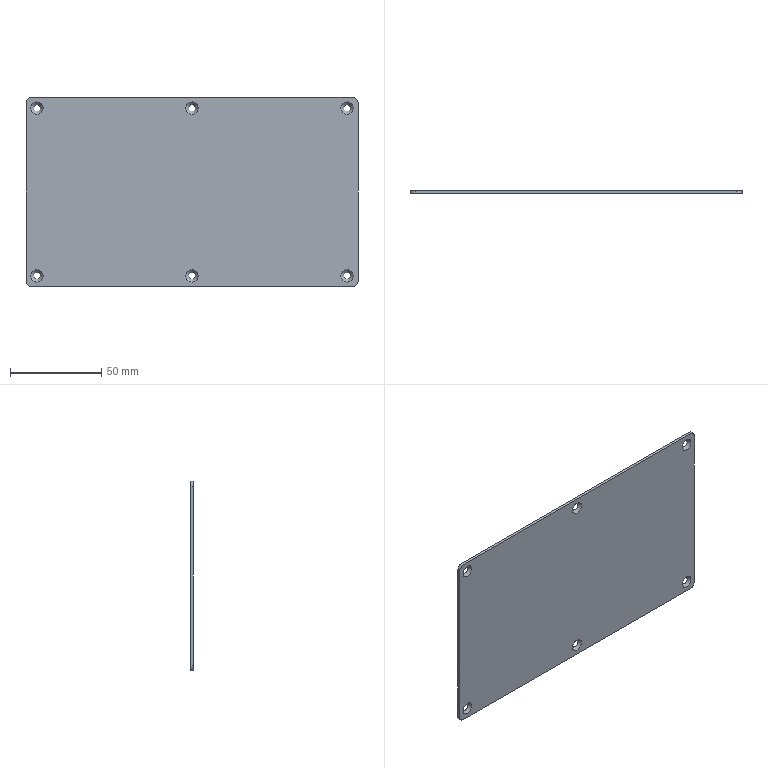Part | NX | 1 solid | 16 faces | box 182 x 1.5 x 104 mm | volume 28183 mm3 | plane 6 | cone 6 | cylinder 4 | commonest cylinder face diameters 6 x4
STEP:
#1=CARTESIAN_POINT('',(-85.,1.5,47.86));
#2=VERTEX_POINT('',#1);
#3=CARTESIAN_POINT('',(-85.,1.5,46.));
#4=DIRECTION('',(0.,1.,0.));
#5=DIRECTION('',(0.,0.,1.));
#6=AXIS2_PLACEMENT_3D('',#3,#4,#5);
#7=CIRCLE('',#6,1.86);
#8=EDGE_CURVE('',#2,#2,#7,.T.);
#9=ORIENTED_EDGE('',*,*,#8,.F.);
#10=EDGE_LOOP('',(#9));
#11=FACE_BOUND('',#10,.T.);
#12=CARTESIAN_POINT('',(-85.,1.5,-44.14));
#13=VERTEX_POINT('',#12);
#14=CARTESIAN_POINT('',(-85.,1.5,-46.));
#15=DIRECTION('',(0.,1.,0.));
#16=DIRECTION('',(0.,0.,1.));
#17=AXIS2_PLACEMENT_3D('',#14,#15,#16);
#18=CIRCLE('',#17,1.86);
#19=EDGE_CURVE('',#13,#13,#18,.T.);
#20=ORIENTED_EDGE('',*,*,#19,.F.);
#21=EDGE_LOOP('',(#20));
#22=FACE_BOUND('',#21,.T.);
#23=CARTESIAN_POINT('',(85.,1.5,-44.14));
#24=VERTEX_POINT('',#23);
#25=CARTESIAN_POINT('',(85.,1.5,-46.));
#26=DIRECTION('',(0.,1.,0.));
#27=DIRECTION('',(0.,0.,1.));
#28=AXIS2_PLACEMENT_3D('',#25,#26,#27);
#29=CIRCLE('',#28,1.86);
#30=EDGE_CURVE('',#24,#24,#29,.T.);
#31=ORIENTED_EDGE('',*,*,#30,.F.);
#32=EDGE_LOOP('',(#31));
#33=FACE_BOUND('',#32,.T.);
#34=CARTESIAN_POINT('',(0.,1.5,-44.14));
#35=VERTEX_POINT('',#34);
#36=CARTESIAN_POINT('',(0.,1.5,-46.));
#37=DIRECTION('',(0.,1.,0.));
#38=DIRECTION('',(0.,0.,1.));
#39=AXIS2_PLACEMENT_3D('',#36,#37,#38);
#40=CIRCLE('',#39,1.86);
#41=EDGE_CURVE('',#35,#35,#40,.T.);
#42=ORIENTED_EDGE('',*,*,#41,.F.);
#43=EDGE_LOOP('',(#42));
#44=FACE_BOUND('',#43,.T.);
#45=CARTESIAN_POINT('',(-88.,1.5,52.));
#46=VERTEX_POINT('',#45);
#47=CARTESIAN_POINT('',(88.,1.5,52.));
#48=VERTEX_POINT('',#47);
#49=CARTESIAN_POINT('',(-91.,1.5,52.));
#50=DIRECTION('',(1.,0.,0.));
#51=VECTOR('',#50,1000.);
#52=LINE('',#49,#51);
#53=EDGE_CURVE('',#46,#48,#52,.T.);
#54=ORIENTED_EDGE('',*,*,#53,.T.);
#55=CARTESIAN_POINT('',(91.,1.5,49.));
#56=VERTEX_POINT('',#55);
#57=CARTESIAN_POINT('',(88.,1.5,49.));
#58=DIRECTION('',(0.,1.,0.));
#59=DIRECTION('',(0.,0.,1.));
#60=AXIS2_PLACEMENT_3D('',#57,#58,#59);
#61=CIRCLE('',#60,3.);
#62=EDGE_CURVE('',#48,#56,#61,.T.);
#63=ORIENTED_EDGE('',*,*,#62,.T.);
#64=CARTESIAN_POINT('',(91.,1.5,-49.));
#65=VERTEX_POINT('',#64);
#66=CARTESIAN_POINT('',(91.,1.5,-52.));
#67=DIRECTION('',(0.,0.,-1.));
#68=VECTOR('',#67,1000.);
#69=LINE('',#66,#68);
#70=EDGE_CURVE('',#56,#65,#69,.T.);
#71=ORIENTED_EDGE('',*,*,#70,.T.);
#72=CARTESIAN_POINT('',(88.,1.5,-52.));
#73=VERTEX_POINT('',#72);
#74=CARTESIAN_POINT('',(88.,1.5,-49.));
#75=DIRECTION('',(0.,1.,0.));
#76=DIRECTION('',(0.,0.,1.));
#77=AXIS2_PLACEMENT_3D('',#74,#75,#76);
#78=CIRCLE('',#77,3.);
#79=EDGE_CURVE('',#65,#73,#78,.T.);
#80=ORIENTED_EDGE('',*,*,#79,.T.);
#81=CARTESIAN_POINT('',(-88.,1.5,-52.));
#82=VERTEX_POINT('',#81);
#83=CARTESIAN_POINT('',(-91.,1.5,-52.));
#84=DIRECTION('',(-1.,0.,0.));
#85=VECTOR('',#84,1000.);
#86=LINE('',#83,#85);
#87=EDGE_CURVE('',#73,#82,#86,.T.);
#88=ORIENTED_EDGE('',*,*,#87,.T.);
#89=CARTESIAN_POINT('',(-91.,1.5,-49.));
#90=VERTEX_POINT('',#89);
#91=CARTESIAN_POINT('',(-88.,1.5,-49.));
#92=DIRECTION('',(0.,1.,0.));
#93=DIRECTION('',(0.,0.,1.));
#94=AXIS2_PLACEMENT_3D('',#91,#92,#93);
#95=CIRCLE('',#94,3.);
#96=EDGE_CURVE('',#82,#90,#95,.T.);
#97=ORIENTED_EDGE('',*,*,#96,.T.);
#98=CARTESIAN_POINT('',(-91.,1.5,49.));
#99=VERTEX_POINT('',#98);
#100=CARTESIAN_POINT('',(-91.,1.5,-52.));
#101=DIRECTION('',(0.,0.,1.));
#102=VECTOR('',#101,1000.);
#103=LINE('',#100,#102);
#104=EDGE_CURVE('',#90,#99,#103,.T.);
#105=ORIENTED_EDGE('',*,*,#104,.T.);
#106=CARTESIAN_POINT('',(-88.,1.5,49.));
#107=DIRECTION('',(0.,1.,0.));
#108=DIRECTION('',(0.,0.,1.));
#109=AXIS2_PLACEMENT_3D('',#106,#107,#108);
#110=CIRCLE('',#109,3.);
#111=EDGE_CURVE('',#99,#46,#110,.T.);
#112=ORIENTED_EDGE('',*,*,#111,.T.);
#113=EDGE_LOOP('',(#54,#63,#71,#80,#88,#97,#105,#112));
#114=FACE_BOUND('',#113,.T.);
#115=CARTESIAN_POINT('',(0.,1.5,47.86));
#116=VERTEX_POINT('',#115);
#117=CARTESIAN_POINT('',(0.,1.5,46.));
#118=DIRECTION('',(0.,1.,0.));
#119=DIRECTION('',(0.,0.,1.));
#120=AXIS2_PLACEMENT_3D('',#117,#118,#119);
#121=CIRCLE('',#120,1.86);
#122=EDGE_CURVE('',#116,#116,#121,.T.);
#123=ORIENTED_EDGE('',*,*,#122,.F.);
#124=EDGE_LOOP('',(#123));
#125=FACE_BOUND('',#124,.T.);
#126=CARTESIAN_POINT('',(85.,1.5,47.86));
#127=VERTEX_POINT('',#126);
#128=CARTESIAN_POINT('',(85.,1.5,46.));
#129=DIRECTION('',(0.,1.,0.));
#130=DIRECTION('',(0.,0.,1.));
#131=AXIS2_PLACEMENT_3D('',#128,#129,#130);
#132=CIRCLE('',#131,1.86);
#133=EDGE_CURVE('',#127,#127,#132,.T.);
#134=ORIENTED_EDGE('',*,*,#133,.F.);
#135=EDGE_LOOP('',(#134));
#136=FACE_BOUND('',#135,.T.);
#137=CARTESIAN_POINT('',(0.,1.5,0.));
#138=DIRECTION('',(0.,1.,0.));
#139=DIRECTION('',(0.,0.,1.));
#140=AXIS2_PLACEMENT_3D('',#137,#138,#139);
#141=PLANE('',#140);
#142=ADVANCED_FACE('',(#11,#22,#33,#44,#114,#125,#136),#141,.T.);
#143=ORIENTED_EDGE('',*,*,#70,.F.);
#144=CARTESIAN_POINT('',(91.,0.,49.));
#145=VERTEX_POINT('',#144);
#146=CARTESIAN_POINT('',(91.,1.5,49.));
#147=DIRECTION('',(0.,-1.,0.));
#148=VECTOR('',#147,1000.);
#149=LINE('',#146,#148);
#150=EDGE_CURVE('',#56,#145,#149,.T.);
#151=ORIENTED_EDGE('',*,*,#150,.T.);
#152=CARTESIAN_POINT('',(91.,0.,-49.));
#153=VERTEX_POINT('',#152);
#154=CARTESIAN_POINT('',(91.,0.,-52.));
#155=DIRECTION('',(0.,0.,-1.));
#156=VECTOR('',#155,1000.);
#157=LINE('',#154,#156);
#158=EDGE_CURVE('',#145,#153,#157,.T.);
#159=ORIENTED_EDGE('',*,*,#158,.T.);
#160=CARTESIAN_POINT('',(91.,1.5,-49.));
#161=DIRECTION('',(0.,-1.,0.));
#162=VECTOR('',#161,1000.);
#163=LINE('',#160,#162);
#164=EDGE_CURVE('',#153,#65,#163,.F.);
#165=ORIENTED_EDGE('',*,*,#164,.T.);
#166=EDGE_LOOP('',(#143,#151,#159,#165));
#167=FACE_BOUND('',#166,.T.);
#168=CARTESIAN_POINT('',(91.,1.5,-52.));
#169=DIRECTION('',(-1.,0.,0.));
#170=DIRECTION('',(0.,0.,1.));
#171=AXIS2_PLACEMENT_3D('',#168,#169,#170);
#172=PLANE('',#171);
#173=ADVANCED_FACE('',(#167),#172,.F.);
#174=ORIENTED_EDGE('',*,*,#87,.F.);
#175=CARTESIAN_POINT('',(88.,0.,-52.));
#176=VERTEX_POINT('',#175);
#177=CARTESIAN_POINT('',(88.,1.5,-52.));
#178=DIRECTION('',(0.,-1.,0.));
#179=VECTOR('',#178,1000.);
#180=LINE('',#177,#179);
#181=EDGE_CURVE('',#73,#176,#180,.T.);
#182=ORIENTED_EDGE('',*,*,#181,.T.);
#183=CARTESIAN_POINT('',(-88.,0.,-52.));
#184=VERTEX_POINT('',#183);
#185=CARTESIAN_POINT('',(-91.,0.,-52.));
#186=DIRECTION('',(-1.,0.,0.));
#187=VECTOR('',#186,1000.);
#188=LINE('',#185,#187);
#189=EDGE_CURVE('',#176,#184,#188,.T.);
#190=ORIENTED_EDGE('',*,*,#189,.T.);
#191=CARTESIAN_POINT('',(-88.,1.5,-52.));
#192=DIRECTION('',(0.,-1.,0.));
#193=VECTOR('',#192,1000.);
#194=LINE('',#191,#193);
#195=EDGE_CURVE('',#184,#82,#194,.F.);
#196=ORIENTED_EDGE('',*,*,#195,.T.);
#197=EDGE_LOOP('',(#174,#182,#190,#196));
#198=FACE_BOUND('',#197,.T.);
#199=CARTESIAN_POINT('',(-91.,1.5,-52.));
#200=DIRECTION('',(0.,0.,1.));
#201=DIRECTION('',(1.,0.,0.));
#202=AXIS2_PLACEMENT_3D('',#199,#200,#201);
#203=PLANE('',#202);
#204=ADVANCED_FACE('',(#198),#203,.F.);
#205=CARTESIAN_POINT('',(-91.,0.,-49.));
#206=VERTEX_POINT('',#205);
#207=CARTESIAN_POINT('',(-91.,0.,49.));
#208=VERTEX_POINT('',#207);
#209=CARTESIAN_POINT('',(-91.,0.,-52.));
#210=DIRECTION('',(0.,0.,1.));
#211=VECTOR('',#210,1000.);
#212=LINE('',#209,#211);
#213=EDGE_CURVE('',#206,#208,#212,.T.);
#214=ORIENTED_EDGE('',*,*,#213,.T.);
#215=CARTESIAN_POINT('',(-91.,1.5,49.));
#216=DIRECTION('',(0.,-1.,0.));
#217=VECTOR('',#216,1000.);
#218=LINE('',#215,#217);
#219=EDGE_CURVE('',#208,#99,#218,.F.);
#220=ORIENTED_EDGE('',*,*,#219,.T.);
#221=ORIENTED_EDGE('',*,*,#104,.F.);
#222=CARTESIAN_POINT('',(-91.,1.5,-49.));
#223=DIRECTION('',(0.,-1.,0.));
#224=VECTOR('',#223,1000.);
#225=LINE('',#222,#224);
#226=EDGE_CURVE('',#90,#206,#225,.T.);
#227=ORIENTED_EDGE('',*,*,#226,.T.);
#228=EDGE_LOOP('',(#214,#220,#221,#227));
#229=FACE_BOUND('',#228,.T.);
#230=CARTESIAN_POINT('',(-91.,1.5,-52.));
#231=DIRECTION('',(1.,0.,0.));
#232=DIRECTION('',(0.,0.,-1.));
#233=AXIS2_PLACEMENT_3D('',#230,#231,#232);
#234=PLANE('',#233);
#235=ADVANCED_FACE('',(#229),#234,.F.);
#236=CARTESIAN_POINT('',(-88.,0.,52.));
#237=VERTEX_POINT('',#236);
#238=CARTESIAN_POINT('',(88.,0.,52.));
#239=VERTEX_POINT('',#238);
#240=CARTESIAN_POINT('',(-91.,0.,52.));
#241=DIRECTION('',(1.,0.,0.));
#242=VECTOR('',#241,1000.);
#243=LINE('',#240,#242);
#244=EDGE_CURVE('',#237,#239,#243,.T.);
#245=ORIENTED_EDGE('',*,*,#244,.T.);
#246=CARTESIAN_POINT('',(88.,1.5,52.));
#247=DIRECTION('',(0.,-1.,0.));
#248=VECTOR('',#247,1000.);
#249=LINE('',#246,#248);
#250=EDGE_CURVE('',#239,#48,#249,.F.);
#251=ORIENTED_EDGE('',*,*,#250,.T.);
#252=ORIENTED_EDGE('',*,*,#53,.F.);
#253=CARTESIAN_POINT('',(-88.,1.5,52.));
#254=DIRECTION('',(0.,-1.,0.));
#255=VECTOR('',#254,1000.);
#256=LINE('',#253,#255);
#257=EDGE_CURVE('',#46,#237,#256,.T.);
#258=ORIENTED_EDGE('',*,*,#257,.T.);
#259=EDGE_LOOP('',(#245,#251,#252,#258));
#260=FACE_BOUND('',#259,.T.);
#261=CARTESIAN_POINT('',(-91.,1.5,52.));
#262=DIRECTION('',(0.,0.,-1.));
#263=DIRECTION('',(-1.,0.,0.));
#264=AXIS2_PLACEMENT_3D('',#261,#262,#263);
#265=PLANE('',#264);
#266=ADVANCED_FACE('',(#260),#265,.F.);
#267=CARTESIAN_POINT('',(-85.,0.,42.64));
#268=VERTEX_POINT('',#267);
#269=CARTESIAN_POINT('',(-85.,0.,46.));
#270=DIRECTION('',(0.,-1.,0.));
#271=DIRECTION('',(0.,0.,-1.));
#272=AXIS2_PLACEMENT_3D('',#269,#270,#271);
#273=CIRCLE('',#272,3.36);
#274=EDGE_CURVE('',#268,#268,#273,.T.);
#275=ORIENTED_EDGE('',*,*,#274,.F.);
#276=EDGE_LOOP('',(#275));
#277=FACE_BOUND('',#276,.T.);
#278=CARTESIAN_POINT('',(-85.,0.,-49.36));
#279=VERTEX_POINT('',#278);
#280=CARTESIAN_POINT('',(-85.,0.,-46.));
#281=DIRECTION('',(0.,-1.,0.));
#282=DIRECTION('',(0.,0.,-1.));
#283=AXIS2_PLACEMENT_3D('',#280,#281,#282);
#284=CIRCLE('',#283,3.36);
#285=EDGE_CURVE('',#279,#279,#284,.T.);
#286=ORIENTED_EDGE('',*,*,#285,.F.);
#287=EDGE_LOOP('',(#286));
#288=FACE_BOUND('',#287,.T.);
#289=CARTESIAN_POINT('',(85.,0.,42.64));
#290=VERTEX_POINT('',#289);
#291=CARTESIAN_POINT('',(85.,0.,46.));
#292=DIRECTION('',(0.,-1.,0.));
#293=DIRECTION('',(0.,0.,-1.));
#294=AXIS2_PLACEMENT_3D('',#291,#292,#293);
#295=CIRCLE('',#294,3.36);
#296=EDGE_CURVE('',#290,#290,#295,.T.);
#297=ORIENTED_EDGE('',*,*,#296,.F.);
#298=EDGE_LOOP('',(#297));
#299=FACE_BOUND('',#298,.T.);
#300=CARTESIAN_POINT('',(85.,0.,-49.36));
#301=VERTEX_POINT('',#300);
#302=CARTESIAN_POINT('',(85.,0.,-46.));
#303=DIRECTION('',(0.,-1.,0.));
#304=DIRECTION('',(0.,0.,-1.));
#305=AXIS2_PLACEMENT_3D('',#302,#303,#304);
#306=CIRCLE('',#305,3.36);
#307=EDGE_CURVE('',#301,#301,#306,.T.);
#308=ORIENTED_EDGE('',*,*,#307,.F.);
#309=EDGE_LOOP('',(#308));
#310=FACE_BOUND('',#309,.T.);
#311=CARTESIAN_POINT('',(0.,0.,-49.36));
#312=VERTEX_POINT('',#311);
#313=CARTESIAN_POINT('',(0.,0.,-46.));
#314=DIRECTION('',(0.,-1.,0.));
#315=DIRECTION('',(0.,0.,-1.));
#316=AXIS2_PLACEMENT_3D('',#313,#314,#315);
#317=CIRCLE('',#316,3.36);
#318=EDGE_CURVE('',#312,#312,#317,.T.);
#319=ORIENTED_EDGE('',*,*,#318,.F.);
#320=EDGE_LOOP('',(#319));
#321=FACE_BOUND('',#320,.T.);
#322=CARTESIAN_POINT('',(0.,0.,42.64));
#323=VERTEX_POINT('',#322);
#324=CARTESIAN_POINT('',(0.,0.,46.));
#325=DIRECTION('',(0.,-1.,0.));
#326=DIRECTION('',(0.,0.,-1.));
#327=AXIS2_PLACEMENT_3D('',#324,#325,#326);
#328=CIRCLE('',#327,3.36);
#329=EDGE_CURVE('',#323,#323,#328,.T.);
#330=ORIENTED_EDGE('',*,*,#329,.F.);
#331=EDGE_LOOP('',(#330));
#332=FACE_BOUND('',#331,.T.);
#333=ORIENTED_EDGE('',*,*,#158,.F.);
#334=CARTESIAN_POINT('',(88.,0.,49.));
#335=DIRECTION('',(0.,1.,0.));
#336=DIRECTION('',(0.,0.,1.));
#337=AXIS2_PLACEMENT_3D('',#334,#335,#336);
#338=CIRCLE('',#337,3.);
#339=EDGE_CURVE('',#145,#239,#338,.F.);
#340=ORIENTED_EDGE('',*,*,#339,.T.);
#341=ORIENTED_EDGE('',*,*,#244,.F.);
#342=CARTESIAN_POINT('',(-88.,0.,49.));
#343=DIRECTION('',(0.,1.,0.));
#344=DIRECTION('',(0.,0.,1.));
#345=AXIS2_PLACEMENT_3D('',#342,#343,#344);
#346=CIRCLE('',#345,3.);
#347=EDGE_CURVE('',#237,#208,#346,.F.);
#348=ORIENTED_EDGE('',*,*,#347,.T.);
#349=ORIENTED_EDGE('',*,*,#213,.F.);
#350=CARTESIAN_POINT('',(-88.,0.,-49.));
#351=DIRECTION('',(0.,1.,0.));
#352=DIRECTION('',(0.,0.,1.));
#353=AXIS2_PLACEMENT_3D('',#350,#351,#352);
#354=CIRCLE('',#353,3.);
#355=EDGE_CURVE('',#206,#184,#354,.F.);
#356=ORIENTED_EDGE('',*,*,#355,.T.);
#357=ORIENTED_EDGE('',*,*,#189,.F.);
#358=CARTESIAN_POINT('',(88.,0.,-49.));
#359=DIRECTION('',(0.,1.,0.));
#360=DIRECTION('',(0.,0.,1.));
#361=AXIS2_PLACEMENT_3D('',#358,#359,#360);
#362=CIRCLE('',#361,3.);
#363=EDGE_CURVE('',#176,#153,#362,.F.);
#364=ORIENTED_EDGE('',*,*,#363,.T.);
#365=EDGE_LOOP('',(#333,#340,#341,#348,#349,#356,#357,#364));
#366=FACE_BOUND('',#365,.T.);
#367=CARTESIAN_POINT('',(0.,0.,0.));
#368=DIRECTION('',(0.,1.,0.));
#369=DIRECTION('',(0.,0.,1.));
#370=AXIS2_PLACEMENT_3D('',#367,#368,#369);
#371=PLANE('',#370);
#372=ADVANCED_FACE('',(#277,#288,#299,#310,#321,#332,#366),#371,.F.);
#373=ORIENTED_EDGE('',*,*,#122,.T.);
#374=EDGE_LOOP('',(#373));
#375=FACE_BOUND('',#374,.T.);
#376=ORIENTED_EDGE('',*,*,#329,.T.);
#377=EDGE_LOOP('',(#376));
#378=FACE_BOUND('',#377,.T.);
#379=CARTESIAN_POINT('',(0.,0.,46.));
#380=DIRECTION('',(0.,-1.,0.));
#381=DIRECTION('',(0.,0.,-1.));
#382=AXIS2_PLACEMENT_3D('',#379,#380,#381);
#383=CONICAL_SURFACE('',#382,3.36,0.7854);
#384=ADVANCED_FACE('',(#375,#378),#383,.F.);
#385=ORIENTED_EDGE('',*,*,#41,.T.);
#386=EDGE_LOOP('',(#385));
#387=FACE_BOUND('',#386,.T.);
#388=ORIENTED_EDGE('',*,*,#318,.T.);
#389=EDGE_LOOP('',(#388));
#390=FACE_BOUND('',#389,.T.);
#391=CARTESIAN_POINT('',(0.,0.,-46.));
#392=DIRECTION('',(0.,-1.,0.));
#393=DIRECTION('',(0.,0.,-1.));
#394=AXIS2_PLACEMENT_3D('',#391,#392,#393);
#395=CONICAL_SURFACE('',#394,3.36,0.7854);
#396=ADVANCED_FACE('',(#387,#390),#395,.F.);
#397=ORIENTED_EDGE('',*,*,#30,.T.);
#398=EDGE_LOOP('',(#397));
#399=FACE_BOUND('',#398,.T.);
#400=ORIENTED_EDGE('',*,*,#307,.T.);
#401=EDGE_LOOP('',(#400));
#402=FACE_BOUND('',#401,.T.);
#403=CARTESIAN_POINT('',(85.,0.,-46.));
#404=DIRECTION('',(0.,-1.,0.));
#405=DIRECTION('',(0.,0.,-1.));
#406=AXIS2_PLACEMENT_3D('',#403,#404,#405);
#407=CONICAL_SURFACE('',#406,3.36,0.7854);
#408=ADVANCED_FACE('',(#399,#402),#407,.F.);
#409=ORIENTED_EDGE('',*,*,#133,.T.);
#410=EDGE_LOOP('',(#409));
#411=FACE_BOUND('',#410,.T.);
#412=ORIENTED_EDGE('',*,*,#296,.T.);
#413=EDGE_LOOP('',(#412));
#414=FACE_BOUND('',#413,.T.);
#415=CARTESIAN_POINT('',(85.,0.,46.));
#416=DIRECTION('',(0.,-1.,0.));
#417=DIRECTION('',(0.,0.,-1.));
#418=AXIS2_PLACEMENT_3D('',#415,#416,#417);
#419=CONICAL_SURFACE('',#418,3.36,0.7854);
#420=ADVANCED_FACE('',(#411,#414),#419,.F.);
#421=ORIENTED_EDGE('',*,*,#19,.T.);
#422=EDGE_LOOP('',(#421));
#423=FACE_BOUND('',#422,.T.);
#424=ORIENTED_EDGE('',*,*,#285,.T.);
#425=EDGE_LOOP('',(#424));
#426=FACE_BOUND('',#425,.T.);
#427=CARTESIAN_POINT('',(-85.,0.,-46.));
#428=DIRECTION('',(0.,-1.,0.));
#429=DIRECTION('',(0.,0.,-1.));
#430=AXIS2_PLACEMENT_3D('',#427,#428,#429);
#431=CONICAL_SURFACE('',#430,3.36,0.7854);
#432=ADVANCED_FACE('',(#423,#426),#431,.F.);
#433=ORIENTED_EDGE('',*,*,#8,.T.);
#434=EDGE_LOOP('',(#433));
#435=FACE_BOUND('',#434,.T.);
#436=ORIENTED_EDGE('',*,*,#274,.T.);
#437=EDGE_LOOP('',(#436));
#438=FACE_BOUND('',#437,.T.);
#439=CARTESIAN_POINT('',(-85.,0.,46.));
#440=DIRECTION('',(0.,-1.,0.));
#441=DIRECTION('',(0.,0.,-1.));
#442=AXIS2_PLACEMENT_3D('',#439,#440,#441);
#443=CONICAL_SURFACE('',#442,3.36,0.7854);
#444=ADVANCED_FACE('',(#435,#438),#443,.F.);
#445=ORIENTED_EDGE('',*,*,#62,.F.);
#446=ORIENTED_EDGE('',*,*,#250,.F.);
#447=ORIENTED_EDGE('',*,*,#339,.F.);
#448=ORIENTED_EDGE('',*,*,#150,.F.);
#449=EDGE_LOOP('',(#445,#446,#447,#448));
#450=FACE_BOUND('',#449,.T.);
#451=CARTESIAN_POINT('',(88.,1.5,49.));
#452=DIRECTION('',(0.,-1.,0.));
#453=DIRECTION('',(0.,0.,-1.));
#454=AXIS2_PLACEMENT_3D('',#451,#452,#453);
#455=CYLINDRICAL_SURFACE('',#454,3.);
#456=ADVANCED_FACE('',(#450),#455,.T.);
#457=ORIENTED_EDGE('',*,*,#79,.F.);
#458=ORIENTED_EDGE('',*,*,#164,.F.);
#459=ORIENTED_EDGE('',*,*,#363,.F.);
#460=ORIENTED_EDGE('',*,*,#181,.F.);
#461=EDGE_LOOP('',(#457,#458,#459,#460));
#462=FACE_BOUND('',#461,.T.);
#463=CARTESIAN_POINT('',(88.,1.5,-49.));
#464=DIRECTION('',(0.,-1.,0.));
#465=DIRECTION('',(0.,0.,-1.));
#466=AXIS2_PLACEMENT_3D('',#463,#464,#465);
#467=CYLINDRICAL_SURFACE('',#466,3.);
#468=ADVANCED_FACE('',(#462),#467,.T.);
#469=ORIENTED_EDGE('',*,*,#111,.F.);
#470=ORIENTED_EDGE('',*,*,#219,.F.);
#471=ORIENTED_EDGE('',*,*,#347,.F.);
#472=ORIENTED_EDGE('',*,*,#257,.F.);
#473=EDGE_LOOP('',(#469,#470,#471,#472));
#474=FACE_BOUND('',#473,.T.);
#475=CARTESIAN_POINT('',(-88.,1.5,49.));
#476=DIRECTION('',(0.,-1.,0.));
#477=DIRECTION('',(0.,0.,-1.));
#478=AXIS2_PLACEMENT_3D('',#475,#476,#477);
#479=CYLINDRICAL_SURFACE('',#478,3.);
#480=ADVANCED_FACE('',(#474),#479,.T.);
#481=ORIENTED_EDGE('',*,*,#96,.F.);
#482=ORIENTED_EDGE('',*,*,#195,.F.);
#483=ORIENTED_EDGE('',*,*,#355,.F.);
#484=ORIENTED_EDGE('',*,*,#226,.F.);
#485=EDGE_LOOP('',(#481,#482,#483,#484));
#486=FACE_BOUND('',#485,.T.);
#487=CARTESIAN_POINT('',(-88.,1.5,-49.));
#488=DIRECTION('',(0.,-1.,0.));
#489=DIRECTION('',(0.,0.,-1.));
#490=AXIS2_PLACEMENT_3D('',#487,#488,#489);
#491=CYLINDRICAL_SURFACE('',#490,3.);
#492=ADVANCED_FACE('',(#486),#491,.T.);
#493=CLOSED_SHELL('',(#142,#173,#204,#235,#266,#372,#384,#396,#408,#420,#432,#444,#456,#468,#480,#492));
#494=MANIFOLD_SOLID_BREP('',#493);
#495=(LENGTH_UNIT()NAMED_UNIT(*)SI_UNIT(.MILLI.,.METRE.));
#496=UNCERTAINTY_MEASURE_WITH_UNIT(LENGTH_MEASURE(0.00001),#495,'','');
#497=(NAMED_UNIT(*)PLANE_ANGLE_UNIT()SI_UNIT($,.RADIAN.));
#498=(NAMED_UNIT(*)SI_UNIT($,.STERADIAN.)SOLID_ANGLE_UNIT());
#499=(GEOMETRIC_REPRESENTATION_CONTEXT(3)GLOBAL_UNCERTAINTY_ASSIGNED_CONTEXT((#496))GLOBAL_UNIT_ASSIGNED_CONTEXT((#495,#497,#498))REPRESENTATION_CONTEXT('',''));
#500=ADVANCED_BREP_SHAPE_REPRESENTATION('',(#494),#499);